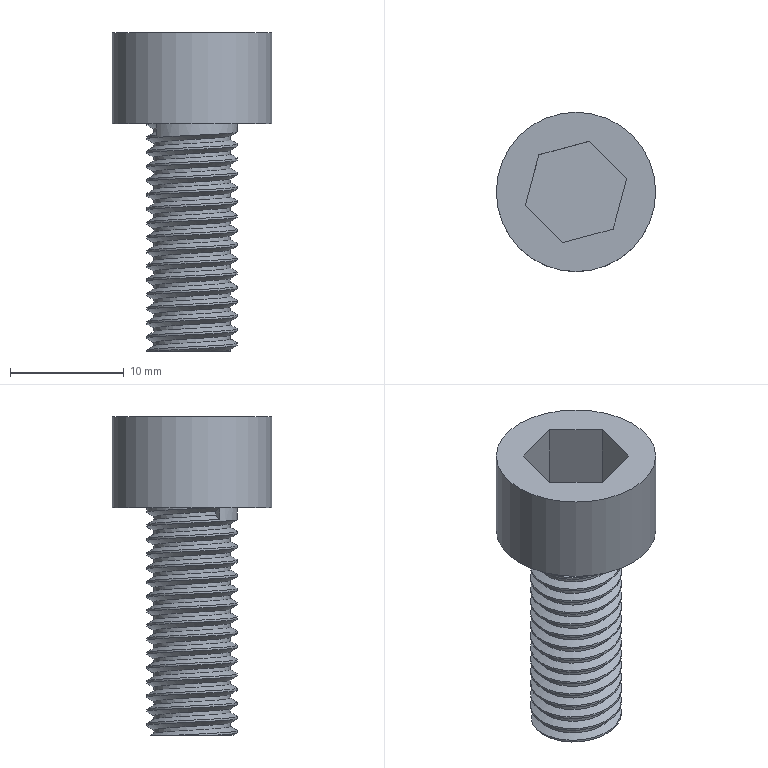Part | NX | features DATUM_CSYS 4, EXTRUDE 3, SKETCH 3, THREADS 1 | 1 solid | 17 faces | box 14 x 14 x 28 mm | volume 1746 mm3 | plane 11 | cylinder 3 | spline 3 | commonest cylinder face diameters 6.75 x1 8 x1 14 x1